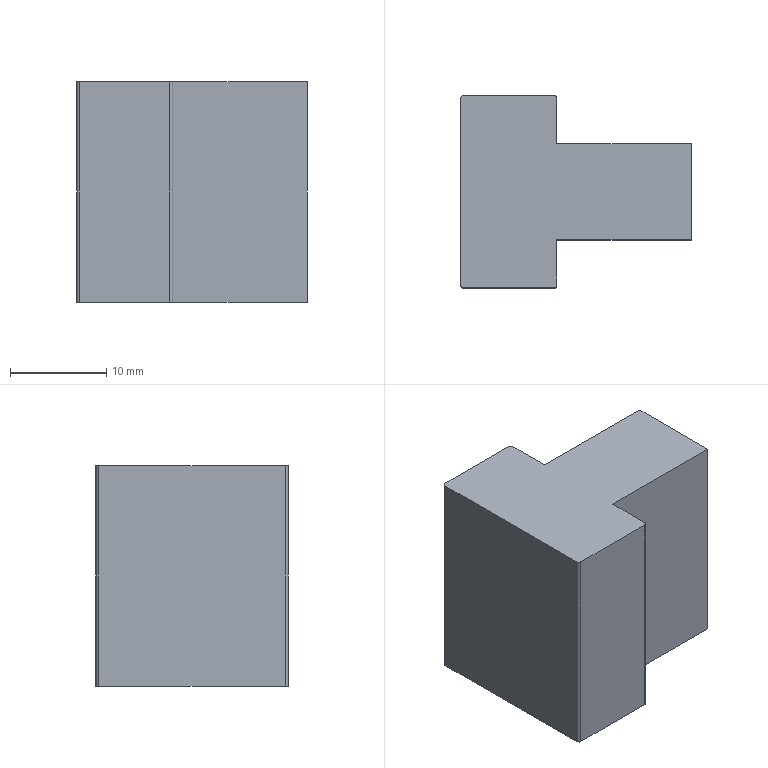Part | STEP file | 200 mesh_id2114 | 1 solid | 14 faces | box 24 x 20 x 22.9 mm | volume 7784 mm3 | plane 10 | cylinder 4 | commonest cylinder face diameters 0.6 x4
STEP:
#1=CARTESIAN_POINT('',(-16836.884,-3950.269,20.));
#2=VERTEX_POINT('',#1);
#3=CARTESIAN_POINT('',(-16836.884,-3960.269,20.));
#4=VERTEX_POINT('',#3);
#5=CARTESIAN_POINT('',(-16836.884,-3964.969,20.));
#6=DIRECTION('',(0.,-1.,0.));
#7=VECTOR('',#6,1.);
#8=LINE('',#5,#7);
#9=EDGE_CURVE('',#2,#4,#8,.T.);
#10=ORIENTED_EDGE('',*,*,#9,.F.);
#11=CARTESIAN_POINT('',(-16836.884,-3950.269,42.9));
#12=VERTEX_POINT('',#11);
#13=CARTESIAN_POINT('',(-16836.884,-3950.269,44.));
#14=DIRECTION('',(0.,0.,-1.));
#15=VECTOR('',#14,1.);
#16=LINE('',#13,#15);
#17=EDGE_CURVE('',#12,#2,#16,.T.);
#18=ORIENTED_EDGE('',*,*,#17,.F.);
#19=CARTESIAN_POINT('',(-16836.884,-3960.269,42.9));
#20=VERTEX_POINT('',#19);
#21=CARTESIAN_POINT('',(-16836.884,-4122.269,42.9));
#22=DIRECTION('',(0.,-1.,0.));
#23=VECTOR('',#22,1.);
#24=LINE('',#21,#23);
#25=EDGE_CURVE('',#12,#20,#24,.T.);
#26=ORIENTED_EDGE('',*,*,#25,.T.);
#27=CARTESIAN_POINT('',(-16836.884,-3960.269,44.));
#28=DIRECTION('',(0.,0.,-1.));
#29=VECTOR('',#28,1.);
#30=LINE('',#27,#29);
#31=EDGE_CURVE('',#20,#4,#30,.T.);
#32=ORIENTED_EDGE('',*,*,#31,.T.);
#33=EDGE_LOOP('',(#10,#18,#26,#32));
#34=FACE_OUTER_BOUND('',#33,.T.);
#35=CARTESIAN_POINT('',(-16836.884,-3950.269,44.));
#36=DIRECTION('',(1.,0.,0.));
#37=DIRECTION('',(0.,1.,0.));
#38=AXIS2_PLACEMENT_3D('',#35,#36,#37);
#39=PLANE('',#38);
#40=ADVANCED_FACE('',(#34),#39,.T.);
#41=CARTESIAN_POINT('',(-16850.884,-3960.269,20.));
#42=VERTEX_POINT('',#41);
#43=CARTESIAN_POINT('',(-16837.884,-3960.269,20.));
#44=DIRECTION('',(-1.,0.,0.));
#45=VECTOR('',#44,1.);
#46=LINE('',#43,#45);
#47=EDGE_CURVE('',#4,#42,#46,.T.);
#48=ORIENTED_EDGE('',*,*,#47,.F.);
#49=ORIENTED_EDGE('',*,*,#31,.F.);
#50=CARTESIAN_POINT('',(-16850.884,-3960.269,42.9));
#51=VERTEX_POINT('',#50);
#52=CARTESIAN_POINT('',(-16925.551,-3960.269,42.9));
#53=DIRECTION('',(-1.,0.,0.));
#54=VECTOR('',#53,1.);
#55=LINE('',#52,#54);
#56=EDGE_CURVE('',#20,#51,#55,.T.);
#57=ORIENTED_EDGE('',*,*,#56,.T.);
#58=CARTESIAN_POINT('',(-16850.884,-3960.269,44.));
#59=DIRECTION('',(0.,0.,-1.));
#60=VECTOR('',#59,1.);
#61=LINE('',#58,#60);
#62=EDGE_CURVE('',#51,#42,#61,.T.);
#63=ORIENTED_EDGE('',*,*,#62,.T.);
#64=EDGE_LOOP('',(#48,#49,#57,#63));
#65=FACE_OUTER_BOUND('',#64,.T.);
#66=CARTESIAN_POINT('',(-16837.884,-3960.269,44.));
#67=DIRECTION('',(0.,-1.,0.));
#68=DIRECTION('',(0.,0.,-1.));
#69=AXIS2_PLACEMENT_3D('',#66,#67,#68);
#70=PLANE('',#69);
#71=ADVANCED_FACE('',(#65),#70,.T.);
#72=CARTESIAN_POINT('',(-16850.884,-3964.969,20.));
#73=VERTEX_POINT('',#72);
#74=CARTESIAN_POINT('',(-16850.884,-3960.269,20.));
#75=DIRECTION('',(0.,-1.,0.));
#76=VECTOR('',#75,1.);
#77=LINE('',#74,#76);
#78=EDGE_CURVE('',#42,#73,#77,.T.);
#79=ORIENTED_EDGE('',*,*,#78,.F.);
#80=ORIENTED_EDGE('',*,*,#62,.F.);
#81=CARTESIAN_POINT('',(-16850.884,-3964.969,42.9));
#82=VERTEX_POINT('',#81);
#83=CARTESIAN_POINT('',(-16850.884,-4122.269,42.9));
#84=DIRECTION('',(0.,-1.,0.));
#85=VECTOR('',#84,1.);
#86=LINE('',#83,#85);
#87=EDGE_CURVE('',#51,#82,#86,.T.);
#88=ORIENTED_EDGE('',*,*,#87,.T.);
#89=CARTESIAN_POINT('',(-16850.884,-3964.969,44.));
#90=DIRECTION('',(0.,0.,-1.));
#91=VECTOR('',#90,1.);
#92=LINE('',#89,#91);
#93=EDGE_CURVE('',#82,#73,#92,.T.);
#94=ORIENTED_EDGE('',*,*,#93,.T.);
#95=EDGE_LOOP('',(#79,#80,#88,#94));
#96=FACE_OUTER_BOUND('',#95,.T.);
#97=CARTESIAN_POINT('',(-16850.884,-3960.269,44.));
#98=DIRECTION('',(1.,0.,0.));
#99=DIRECTION('',(0.,0.,-1.));
#100=AXIS2_PLACEMENT_3D('',#97,#98,#99);
#101=PLANE('',#100);
#102=ADVANCED_FACE('',(#96),#101,.T.);
#103=CARTESIAN_POINT('',(-16851.184,-3965.269,20.));
#104=VERTEX_POINT('',#103);
#105=CARTESIAN_POINT('',(-16851.184,-3964.969,20.));
#106=DIRECTION('',(0.,0.,-1.));
#107=DIRECTION('',(1.,0.,0.));
#108=AXIS2_PLACEMENT_3D('',#105,#106,#107);
#109=CIRCLE('',#108,0.3);
#110=EDGE_CURVE('',#73,#104,#109,.T.);
#111=ORIENTED_EDGE('',*,*,#110,.F.);
#112=ORIENTED_EDGE('',*,*,#93,.F.);
#113=CARTESIAN_POINT('',(-16851.184,-3965.269,42.9));
#114=VERTEX_POINT('',#113);
#115=CARTESIAN_POINT('',(-16851.184,-3964.969,42.9));
#116=DIRECTION('',(0.,0.,-1.));
#117=DIRECTION('',(1.,0.,0.));
#118=AXIS2_PLACEMENT_3D('',#115,#116,#117);
#119=CIRCLE('',#118,0.3);
#120=EDGE_CURVE('',#82,#114,#119,.T.);
#121=ORIENTED_EDGE('',*,*,#120,.T.);
#122=CARTESIAN_POINT('',(-16851.184,-3965.269,44.));
#123=DIRECTION('',(0.,0.,-1.));
#124=VECTOR('',#123,1.);
#125=LINE('',#122,#124);
#126=EDGE_CURVE('',#114,#104,#125,.T.);
#127=ORIENTED_EDGE('',*,*,#126,.T.);
#128=EDGE_LOOP('',(#111,#112,#121,#127));
#129=FACE_OUTER_BOUND('',#128,.T.);
#130=CARTESIAN_POINT('',(-16851.184,-3964.969,44.));
#131=DIRECTION('',(0.,0.,-1.));
#132=DIRECTION('',(-1.,0.,0.));
#133=AXIS2_PLACEMENT_3D('',#130,#131,#132);
#134=CYLINDRICAL_SURFACE('',#133,0.3);
#135=ADVANCED_FACE('',(#129),#134,.T.);
#136=CARTESIAN_POINT('',(-16860.584,-3965.269,20.));
#137=VERTEX_POINT('',#136);
#138=CARTESIAN_POINT('',(-16851.184,-3965.269,20.));
#139=DIRECTION('',(-1.,0.,0.));
#140=VECTOR('',#139,1.);
#141=LINE('',#138,#140);
#142=EDGE_CURVE('',#104,#137,#141,.T.);
#143=ORIENTED_EDGE('',*,*,#142,.F.);
#144=ORIENTED_EDGE('',*,*,#126,.F.);
#145=CARTESIAN_POINT('',(-16860.584,-3965.269,42.9));
#146=VERTEX_POINT('',#145);
#147=CARTESIAN_POINT('',(-16925.551,-3965.269,42.9));
#148=DIRECTION('',(-1.,0.,0.));
#149=VECTOR('',#148,1.);
#150=LINE('',#147,#149);
#151=EDGE_CURVE('',#114,#146,#150,.T.);
#152=ORIENTED_EDGE('',*,*,#151,.T.);
#153=CARTESIAN_POINT('',(-16860.584,-3965.269,44.));
#154=DIRECTION('',(0.,0.,-1.));
#155=VECTOR('',#154,1.);
#156=LINE('',#153,#155);
#157=EDGE_CURVE('',#146,#137,#156,.T.);
#158=ORIENTED_EDGE('',*,*,#157,.T.);
#159=EDGE_LOOP('',(#143,#144,#152,#158));
#160=FACE_OUTER_BOUND('',#159,.T.);
#161=CARTESIAN_POINT('',(-16851.184,-3965.269,44.));
#162=DIRECTION('',(0.,-1.,0.));
#163=DIRECTION('',(0.,0.,-1.));
#164=AXIS2_PLACEMENT_3D('',#161,#162,#163);
#165=PLANE('',#164);
#166=ADVANCED_FACE('',(#160),#165,.T.);
#167=CARTESIAN_POINT('',(-16860.884,-3964.969,20.));
#168=VERTEX_POINT('',#167);
#169=CARTESIAN_POINT('',(-16860.584,-3964.969,20.));
#170=DIRECTION('',(0.,0.,-1.));
#171=DIRECTION('',(1.,0.,0.));
#172=AXIS2_PLACEMENT_3D('',#169,#170,#171);
#173=CIRCLE('',#172,0.3);
#174=EDGE_CURVE('',#137,#168,#173,.T.);
#175=ORIENTED_EDGE('',*,*,#174,.F.);
#176=ORIENTED_EDGE('',*,*,#157,.F.);
#177=CARTESIAN_POINT('',(-16860.884,-3964.969,42.9));
#178=VERTEX_POINT('',#177);
#179=CARTESIAN_POINT('',(-16860.584,-3964.969,42.9));
#180=DIRECTION('',(0.,0.,-1.));
#181=DIRECTION('',(1.,0.,0.));
#182=AXIS2_PLACEMENT_3D('',#179,#180,#181);
#183=CIRCLE('',#182,0.3);
#184=EDGE_CURVE('',#146,#178,#183,.T.);
#185=ORIENTED_EDGE('',*,*,#184,.T.);
#186=CARTESIAN_POINT('',(-16860.884,-3964.969,44.));
#187=DIRECTION('',(0.,0.,-1.));
#188=VECTOR('',#187,1.);
#189=LINE('',#186,#188);
#190=EDGE_CURVE('',#178,#168,#189,.T.);
#191=ORIENTED_EDGE('',*,*,#190,.T.);
#192=EDGE_LOOP('',(#175,#176,#185,#191));
#193=FACE_OUTER_BOUND('',#192,.T.);
#194=CARTESIAN_POINT('',(-16860.584,-3964.969,44.));
#195=DIRECTION('',(0.,0.,-1.));
#196=DIRECTION('',(-1.,0.,0.));
#197=AXIS2_PLACEMENT_3D('',#194,#195,#196);
#198=CYLINDRICAL_SURFACE('',#197,0.3);
#199=ADVANCED_FACE('',(#193),#198,.T.);
#200=CARTESIAN_POINT('',(-16860.884,-3945.569,20.));
#201=VERTEX_POINT('',#200);
#202=CARTESIAN_POINT('',(-16860.884,-3964.969,20.));
#203=DIRECTION('',(0.,1.,0.));
#204=VECTOR('',#203,1.);
#205=LINE('',#202,#204);
#206=EDGE_CURVE('',#168,#201,#205,.T.);
#207=ORIENTED_EDGE('',*,*,#206,.F.);
#208=ORIENTED_EDGE('',*,*,#190,.F.);
#209=CARTESIAN_POINT('',(-16860.884,-3945.569,42.9));
#210=VERTEX_POINT('',#209);
#211=CARTESIAN_POINT('',(-16860.884,-4122.269,42.9));
#212=DIRECTION('',(0.,1.,0.));
#213=VECTOR('',#212,1.);
#214=LINE('',#211,#213);
#215=EDGE_CURVE('',#178,#210,#214,.T.);
#216=ORIENTED_EDGE('',*,*,#215,.T.);
#217=CARTESIAN_POINT('',(-16860.884,-3945.569,44.));
#218=DIRECTION('',(0.,0.,-1.));
#219=VECTOR('',#218,1.);
#220=LINE('',#217,#219);
#221=EDGE_CURVE('',#210,#201,#220,.T.);
#222=ORIENTED_EDGE('',*,*,#221,.T.);
#223=EDGE_LOOP('',(#207,#208,#216,#222));
#224=FACE_OUTER_BOUND('',#223,.T.);
#225=CARTESIAN_POINT('',(-16860.884,-3964.969,44.));
#226=DIRECTION('',(-1.,0.,0.));
#227=DIRECTION('',(0.,0.,1.));
#228=AXIS2_PLACEMENT_3D('',#225,#226,#227);
#229=PLANE('',#228);
#230=ADVANCED_FACE('',(#224),#229,.T.);
#231=CARTESIAN_POINT('',(-16860.584,-3945.269,20.));
#232=VERTEX_POINT('',#231);
#233=CARTESIAN_POINT('',(-16860.584,-3945.569,20.));
#234=DIRECTION('',(0.,0.,-1.));
#235=DIRECTION('',(1.,0.,0.));
#236=AXIS2_PLACEMENT_3D('',#233,#234,#235);
#237=CIRCLE('',#236,0.3);
#238=EDGE_CURVE('',#201,#232,#237,.T.);
#239=ORIENTED_EDGE('',*,*,#238,.F.);
#240=ORIENTED_EDGE('',*,*,#221,.F.);
#241=CARTESIAN_POINT('',(-16860.584,-3945.269,42.9));
#242=VERTEX_POINT('',#241);
#243=CARTESIAN_POINT('',(-16860.584,-3945.569,42.9));
#244=DIRECTION('',(0.,0.,-1.));
#245=DIRECTION('',(1.,0.,0.));
#246=AXIS2_PLACEMENT_3D('',#243,#244,#245);
#247=CIRCLE('',#246,0.3);
#248=EDGE_CURVE('',#210,#242,#247,.T.);
#249=ORIENTED_EDGE('',*,*,#248,.T.);
#250=CARTESIAN_POINT('',(-16860.584,-3945.269,44.));
#251=DIRECTION('',(0.,0.,-1.));
#252=VECTOR('',#251,1.);
#253=LINE('',#250,#252);
#254=EDGE_CURVE('',#242,#232,#253,.T.);
#255=ORIENTED_EDGE('',*,*,#254,.T.);
#256=EDGE_LOOP('',(#239,#240,#249,#255));
#257=FACE_OUTER_BOUND('',#256,.T.);
#258=CARTESIAN_POINT('',(-16860.584,-3945.569,44.));
#259=DIRECTION('',(0.,0.,-1.));
#260=DIRECTION('',(-1.,0.,0.));
#261=AXIS2_PLACEMENT_3D('',#258,#259,#260);
#262=CYLINDRICAL_SURFACE('',#261,0.3);
#263=ADVANCED_FACE('',(#257),#262,.T.);
#264=CARTESIAN_POINT('',(-16851.184,-3945.269,20.));
#265=VERTEX_POINT('',#264);
#266=CARTESIAN_POINT('',(-16860.584,-3945.269,20.));
#267=DIRECTION('',(1.,0.,0.));
#268=VECTOR('',#267,1.);
#269=LINE('',#266,#268);
#270=EDGE_CURVE('',#232,#265,#269,.T.);
#271=ORIENTED_EDGE('',*,*,#270,.F.);
#272=ORIENTED_EDGE('',*,*,#254,.F.);
#273=CARTESIAN_POINT('',(-16851.184,-3945.269,42.9));
#274=VERTEX_POINT('',#273);
#275=CARTESIAN_POINT('',(-16925.551,-3945.269,42.9));
#276=DIRECTION('',(1.,0.,0.));
#277=VECTOR('',#276,1.);
#278=LINE('',#275,#277);
#279=EDGE_CURVE('',#242,#274,#278,.T.);
#280=ORIENTED_EDGE('',*,*,#279,.T.);
#281=CARTESIAN_POINT('',(-16851.184,-3945.269,44.));
#282=DIRECTION('',(0.,0.,-1.));
#283=VECTOR('',#282,1.);
#284=LINE('',#281,#283);
#285=EDGE_CURVE('',#274,#265,#284,.T.);
#286=ORIENTED_EDGE('',*,*,#285,.T.);
#287=EDGE_LOOP('',(#271,#272,#280,#286));
#288=FACE_OUTER_BOUND('',#287,.T.);
#289=CARTESIAN_POINT('',(-16860.584,-3945.269,44.));
#290=DIRECTION('',(0.,1.,0.));
#291=DIRECTION('',(0.,0.,1.));
#292=AXIS2_PLACEMENT_3D('',#289,#290,#291);
#293=PLANE('',#292);
#294=ADVANCED_FACE('',(#288),#293,.T.);
#295=CARTESIAN_POINT('',(-16850.884,-3945.569,20.));
#296=VERTEX_POINT('',#295);
#297=CARTESIAN_POINT('',(-16851.184,-3945.569,20.));
#298=DIRECTION('',(0.,0.,-1.));
#299=DIRECTION('',(1.,0.,0.));
#300=AXIS2_PLACEMENT_3D('',#297,#298,#299);
#301=CIRCLE('',#300,0.3);
#302=EDGE_CURVE('',#265,#296,#301,.T.);
#303=ORIENTED_EDGE('',*,*,#302,.F.);
#304=ORIENTED_EDGE('',*,*,#285,.F.);
#305=CARTESIAN_POINT('',(-16850.884,-3945.569,42.9));
#306=VERTEX_POINT('',#305);
#307=CARTESIAN_POINT('',(-16851.184,-3945.569,42.9));
#308=DIRECTION('',(0.,0.,-1.));
#309=DIRECTION('',(1.,0.,0.));
#310=AXIS2_PLACEMENT_3D('',#307,#308,#309);
#311=CIRCLE('',#310,0.3);
#312=EDGE_CURVE('',#274,#306,#311,.T.);
#313=ORIENTED_EDGE('',*,*,#312,.T.);
#314=CARTESIAN_POINT('',(-16850.884,-3945.569,44.));
#315=DIRECTION('',(0.,0.,-1.));
#316=VECTOR('',#315,1.);
#317=LINE('',#314,#316);
#318=EDGE_CURVE('',#306,#296,#317,.T.);
#319=ORIENTED_EDGE('',*,*,#318,.T.);
#320=EDGE_LOOP('',(#303,#304,#313,#319));
#321=FACE_OUTER_BOUND('',#320,.T.);
#322=CARTESIAN_POINT('',(-16851.184,-3945.569,44.));
#323=DIRECTION('',(0.,0.,-1.));
#324=DIRECTION('',(-1.,0.,0.));
#325=AXIS2_PLACEMENT_3D('',#322,#323,#324);
#326=CYLINDRICAL_SURFACE('',#325,0.3);
#327=ADVANCED_FACE('',(#321),#326,.T.);
#328=CARTESIAN_POINT('',(-16850.884,-3950.269,20.));
#329=VERTEX_POINT('',#328);
#330=CARTESIAN_POINT('',(-16850.884,-3945.569,20.));
#331=DIRECTION('',(0.,-1.,0.));
#332=VECTOR('',#331,1.);
#333=LINE('',#330,#332);
#334=EDGE_CURVE('',#296,#329,#333,.T.);
#335=ORIENTED_EDGE('',*,*,#334,.F.);
#336=ORIENTED_EDGE('',*,*,#318,.F.);
#337=CARTESIAN_POINT('',(-16850.884,-3950.269,42.9));
#338=VERTEX_POINT('',#337);
#339=CARTESIAN_POINT('',(-16850.884,-4122.269,42.9));
#340=DIRECTION('',(0.,-1.,0.));
#341=VECTOR('',#340,1.);
#342=LINE('',#339,#341);
#343=EDGE_CURVE('',#306,#338,#342,.T.);
#344=ORIENTED_EDGE('',*,*,#343,.T.);
#345=CARTESIAN_POINT('',(-16850.884,-3950.269,44.));
#346=DIRECTION('',(0.,0.,-1.));
#347=VECTOR('',#346,1.);
#348=LINE('',#345,#347);
#349=EDGE_CURVE('',#338,#329,#348,.T.);
#350=ORIENTED_EDGE('',*,*,#349,.T.);
#351=EDGE_LOOP('',(#335,#336,#344,#350));
#352=FACE_OUTER_BOUND('',#351,.T.);
#353=CARTESIAN_POINT('',(-16850.884,-3945.569,44.));
#354=DIRECTION('',(1.,0.,0.));
#355=DIRECTION('',(0.,1.,0.));
#356=AXIS2_PLACEMENT_3D('',#353,#354,#355);
#357=PLANE('',#356);
#358=ADVANCED_FACE('',(#352),#357,.T.);
#359=CARTESIAN_POINT('',(-16850.884,-3950.269,20.));
#360=DIRECTION('',(1.,0.,0.));
#361=VECTOR('',#360,1.);
#362=LINE('',#359,#361);
#363=EDGE_CURVE('',#329,#2,#362,.T.);
#364=ORIENTED_EDGE('',*,*,#363,.F.);
#365=ORIENTED_EDGE('',*,*,#349,.F.);
#366=CARTESIAN_POINT('',(-16925.551,-3950.269,42.9));
#367=DIRECTION('',(1.,0.,0.));
#368=VECTOR('',#367,1.);
#369=LINE('',#366,#368);
#370=EDGE_CURVE('',#338,#12,#369,.T.);
#371=ORIENTED_EDGE('',*,*,#370,.T.);
#372=ORIENTED_EDGE('',*,*,#17,.T.);
#373=EDGE_LOOP('',(#364,#365,#371,#372));
#374=FACE_OUTER_BOUND('',#373,.T.);
#375=CARTESIAN_POINT('',(-16850.884,-3950.269,44.));
#376=DIRECTION('',(0.,1.,0.));
#377=DIRECTION('',(0.,0.,1.));
#378=AXIS2_PLACEMENT_3D('',#375,#376,#377);
#379=PLANE('',#378);
#380=ADVANCED_FACE('',(#374),#379,.T.);
#381=ORIENTED_EDGE('',*,*,#25,.F.);
#382=ORIENTED_EDGE('',*,*,#370,.F.);
#383=ORIENTED_EDGE('',*,*,#343,.F.);
#384=ORIENTED_EDGE('',*,*,#312,.F.);
#385=ORIENTED_EDGE('',*,*,#279,.F.);
#386=ORIENTED_EDGE('',*,*,#248,.F.);
#387=ORIENTED_EDGE('',*,*,#215,.F.);
#388=ORIENTED_EDGE('',*,*,#184,.F.);
#389=ORIENTED_EDGE('',*,*,#151,.F.);
#390=ORIENTED_EDGE('',*,*,#120,.F.);
#391=ORIENTED_EDGE('',*,*,#87,.F.);
#392=ORIENTED_EDGE('',*,*,#56,.F.);
#393=EDGE_LOOP('',(#381,#382,#383,#384,#385,#386,#387,#388,#389,#390,#391,#392));
#394=FACE_OUTER_BOUND('',#393,.T.);
#395=CARTESIAN_POINT('',(-16925.551,-4122.269,42.9));
#396=DIRECTION('',(0.,0.,1.));
#397=DIRECTION('',(-1.,0.,0.));
#398=AXIS2_PLACEMENT_3D('',#395,#396,#397);
#399=PLANE('',#398);
#400=ADVANCED_FACE('',(#394),#399,.T.);
#401=ORIENTED_EDGE('',*,*,#9,.T.);
#402=ORIENTED_EDGE('',*,*,#47,.T.);
#403=ORIENTED_EDGE('',*,*,#78,.T.);
#404=ORIENTED_EDGE('',*,*,#110,.T.);
#405=ORIENTED_EDGE('',*,*,#142,.T.);
#406=ORIENTED_EDGE('',*,*,#174,.T.);
#407=ORIENTED_EDGE('',*,*,#206,.T.);
#408=ORIENTED_EDGE('',*,*,#238,.T.);
#409=ORIENTED_EDGE('',*,*,#270,.T.);
#410=ORIENTED_EDGE('',*,*,#302,.T.);
#411=ORIENTED_EDGE('',*,*,#334,.T.);
#412=ORIENTED_EDGE('',*,*,#363,.T.);
#413=EDGE_LOOP('',(#401,#402,#403,#404,#405,#406,#407,#408,#409,#410,#411,#412));
#414=FACE_OUTER_BOUND('',#413,.T.);
#415=CARTESIAN_POINT('',(-16851.184,-3964.969,20.));
#416=DIRECTION('',(0.,0.,-1.));
#417=DIRECTION('',(-1.,0.,0.));
#418=AXIS2_PLACEMENT_3D('',#415,#416,#417);
#419=PLANE('',#418);
#420=ADVANCED_FACE('',(#414),#419,.T.);
#421=CLOSED_SHELL('',(#40,#71,#102,#135,#166,#199,#230,#263,#294,#327,#358,#380,#400,#420));
#422=MANIFOLD_SOLID_BREP('',#421);
#423=(LENGTH_UNIT()NAMED_UNIT(*)SI_UNIT(.MILLI.,.METRE.));
#424=UNCERTAINTY_MEASURE_WITH_UNIT(LENGTH_MEASURE(0.00002),#423,'','');
#425=(NAMED_UNIT(*)PLANE_ANGLE_UNIT()SI_UNIT($,.RADIAN.));
#426=PLANE_ANGLE_MEASURE_WITH_UNIT(PLANE_ANGLE_MEASURE(0.01745),#425);
#427=DIMENSIONAL_EXPONENTS(0.,0.,0.,0.,0.,0.,0.);
#428=(CONVERSION_BASED_UNIT('DEGREE',#426)NAMED_UNIT(#427)PLANE_ANGLE_UNIT());
#429=(NAMED_UNIT(*)SI_UNIT($,.STERADIAN.)SOLID_ANGLE_UNIT());
#430=(GEOMETRIC_REPRESENTATION_CONTEXT(3)GLOBAL_UNCERTAINTY_ASSIGNED_CONTEXT((#424))GLOBAL_UNIT_ASSIGNED_CONTEXT((#423,#428,#429))REPRESENTATION_CONTEXT('',''));
#431=ADVANCED_BREP_SHAPE_REPRESENTATION('',(#422),#430);